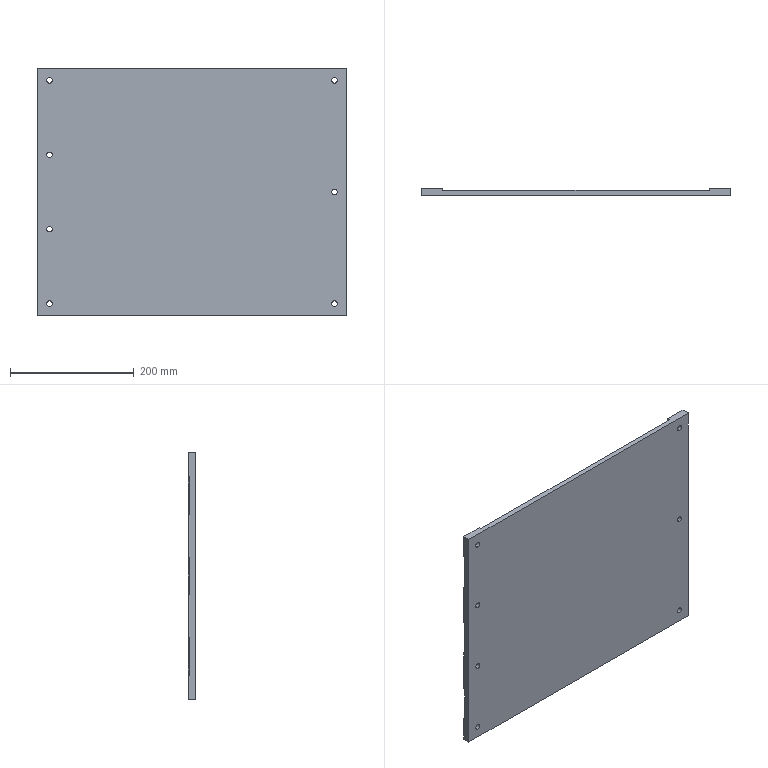Part | SolidWorks | features ICE 4, HoleWzd 2, Extrusion 1, Fillet 1 | 1 solid | 56 faces | box 500 x 11.75 x 400 mm | volume 1689259 mm3 | plane 22 | cylinder 20 | cone 14 | commonest cylinder face diameters 9 x14 10 x6